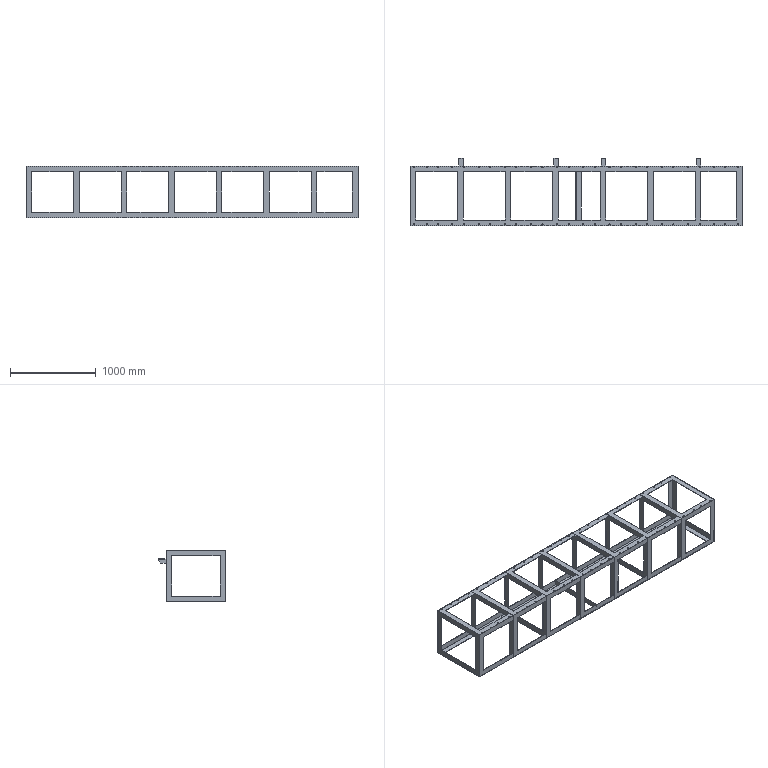Part | STEP file | KHUNG SUON MAY DAP 3660 | 1 solid | 310 faces | box 3868 x 784 x 600 mm | volume 15834108 mm3 | plane 186 | cylinder 124 | commonest cylinder face diameters 13 x104 18 x20